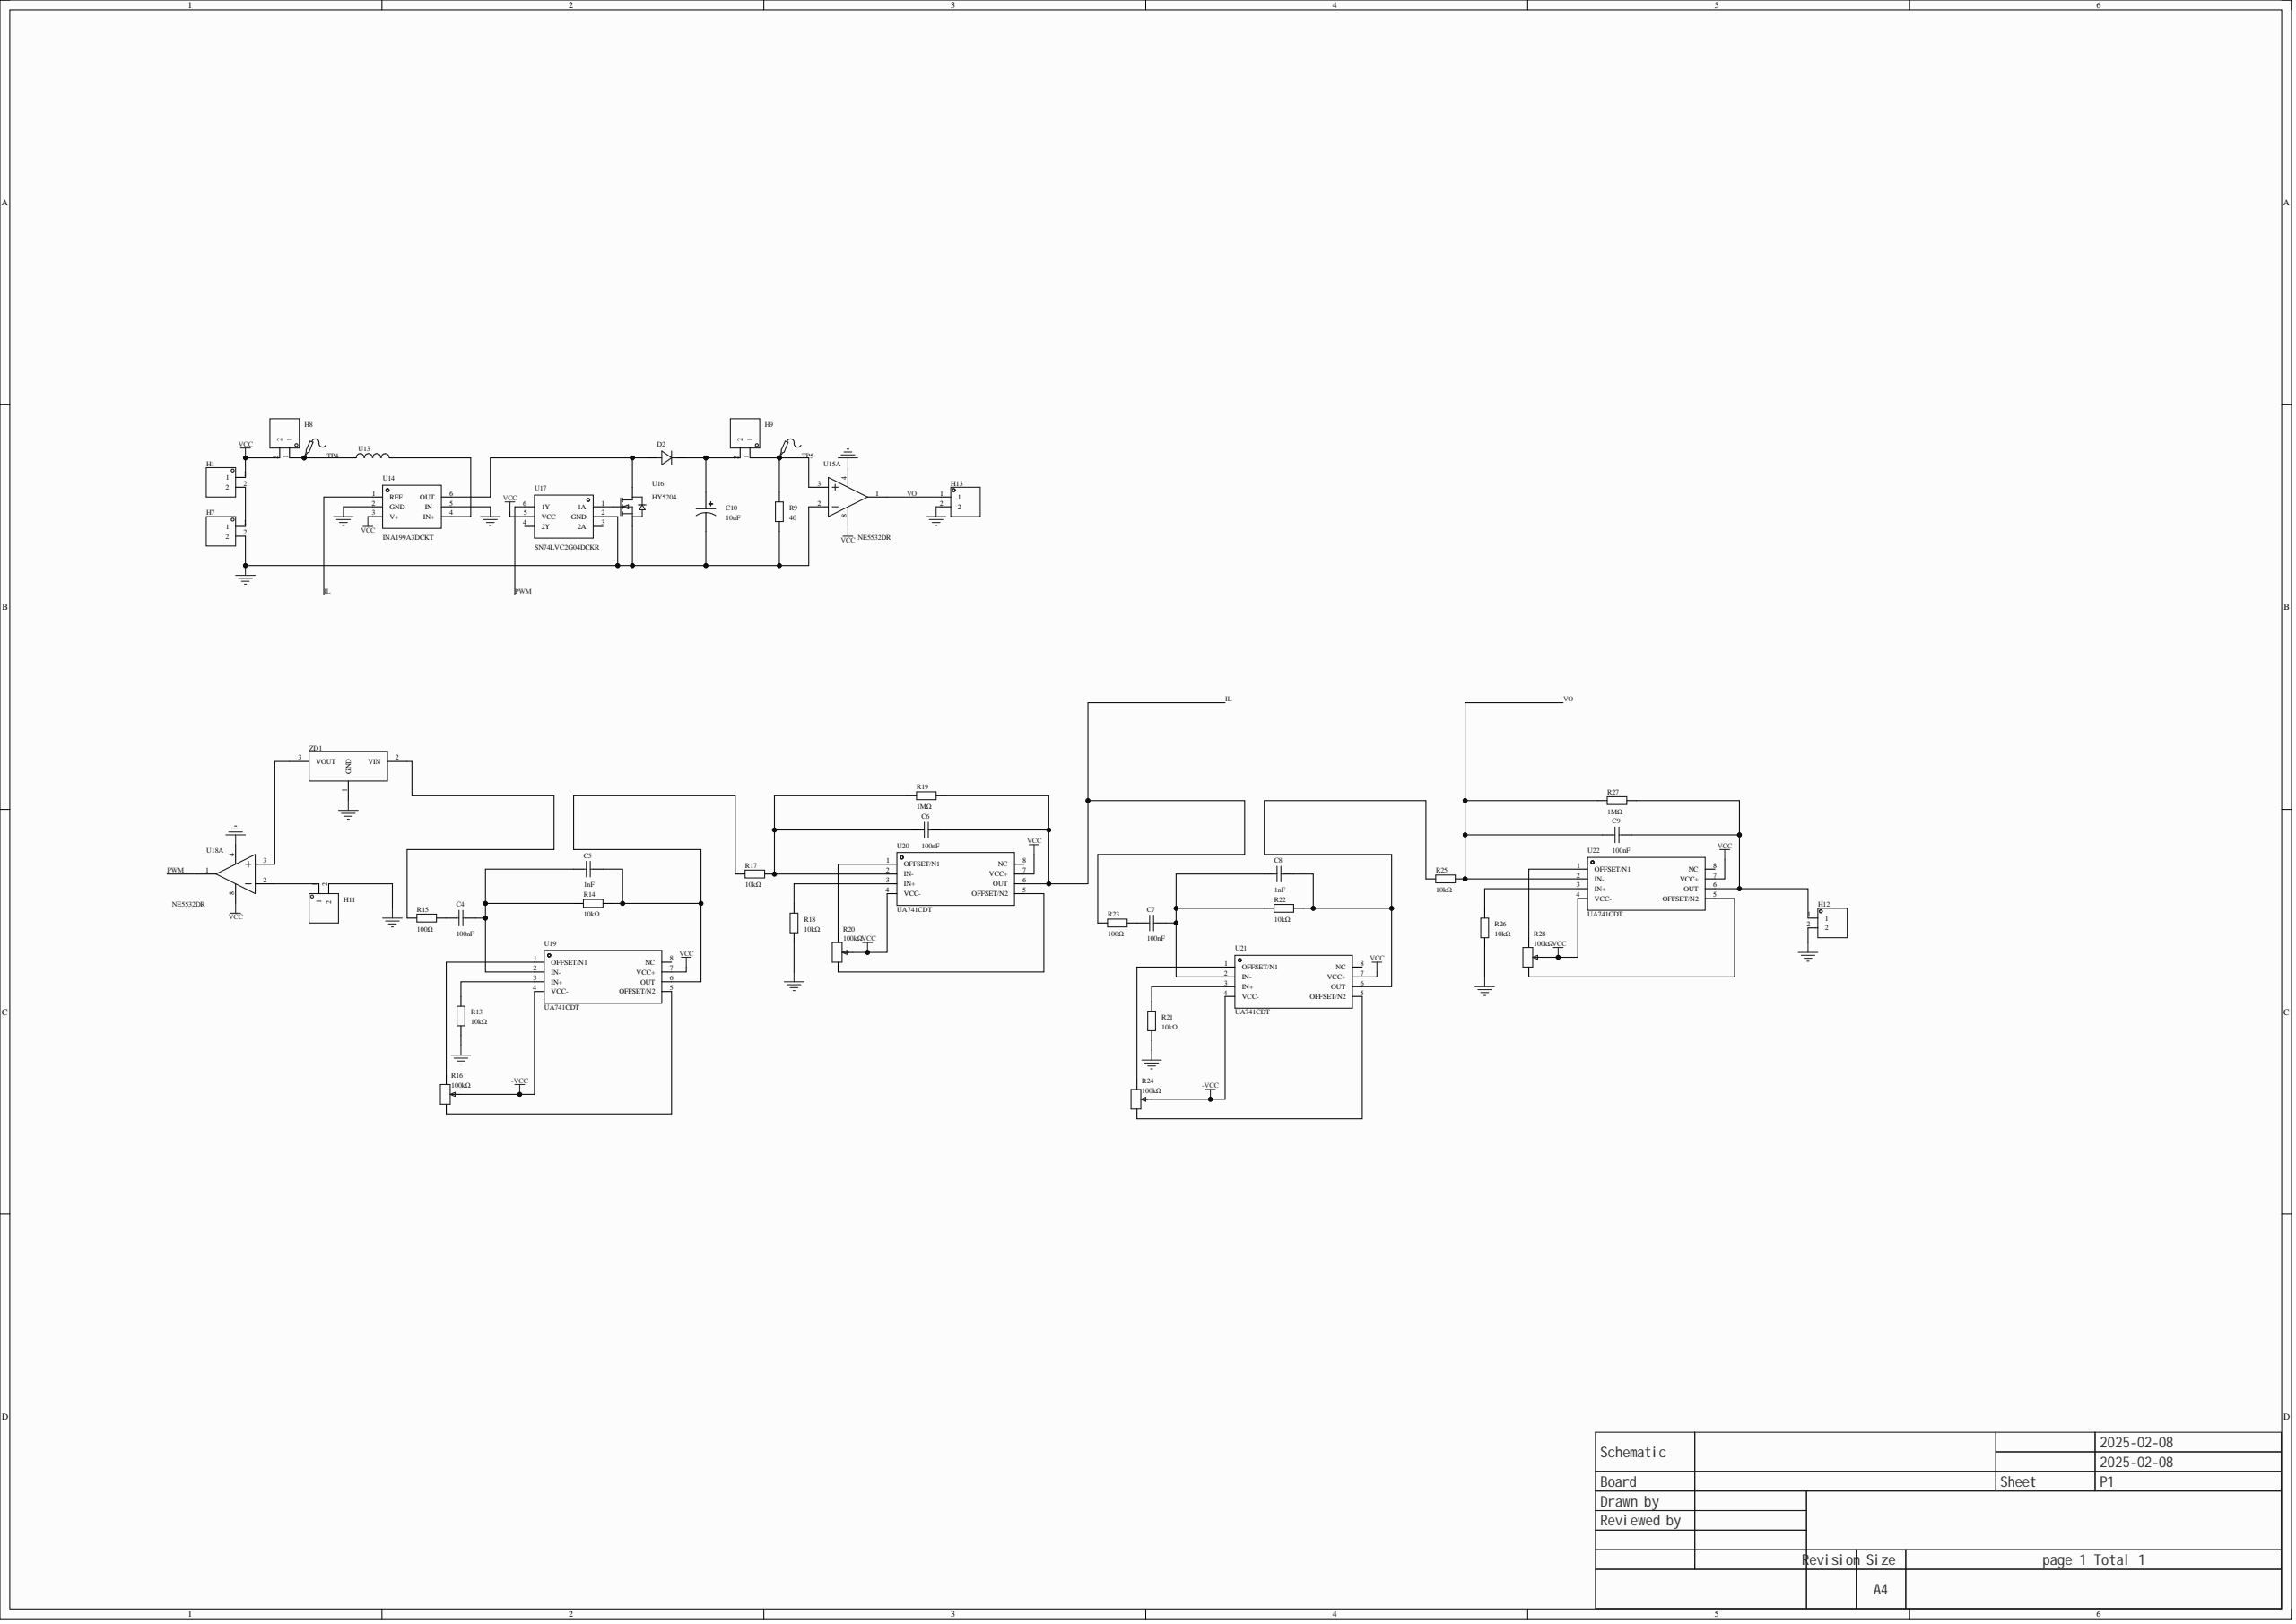Circuit board | Altium Designer | 45 parts | 36 nets
Bill of materials:
Comment,Description,Designator,Footprint,LibRef,Quantity
"100nF","Capacitance: 100nF; Tolerance: ±10%; Rated voltage: 50V; Dielectric (temperature coefficient): X7R;","C4, C6, C7, C9","C0805","CC0805KRX7R9BB104","4"
"1nF","Capacitance: 100nF; Tolerance: ±10%; Rated voltage: 50V; Dielectric (temperature coefficient): X7R;","C5, C8","C0805","CC0805KRX7R9BB104","2"
"10uF","Capacitance: 10uF; Tolerance: ±20%; Rated voltage: 10V; Ripple current: 16mA@120Hz;","C10","CAP-TH_BD4.0-P1.50-D0.8-FD","10MS510MEFC4X5","1"
"","","D2","DO_1N4007","D_1N4007A","1"
"","","H1, H7, H8, H9, H11, H12, H13","HDR-TH_2P-P2.54-V-M-1","HDR-M_2.54_1x2P","7"
"40","","R9","Res_1/4W","Res_AXIAL-1/4W","1"
"10kΩ","Resistor type: thick film resistor; Resistance: 10kΩ; Tolerance: ±1%; Power: 125mW; Max working voltage: 150V; Temperature coefficient: ±100ppm/?;","R13, R14, R17, R18, R21, R22, R25, R26","R0805","0805W8F1002T5E_C17414","8"
"100Ω","Resistor type: thick film resistor; Resistance: 10kΩ; Tolerance: ±1%; Power: 125mW; Max working voltage: 150V; Temperature coefficient: ±100ppm/?;","R15, R23","R0805","0805W8F1002T5E_C17414","2"
"100kΩ","Resistance: 200Ω; Tolerance: ±25%;","R16, R20, R24, R28","RES-ADJ-SMD_VG039NCH","VG039NCHXTB201","4"
"1MΩ","Resistor type: thick film resistor; Resistance: 10kΩ; Tolerance: ±1%; Power: 125mW; Max working voltage: 150V; Temperature coefficient: ±100ppm/?;","R19, R27","R0805","0805W8F1002T5E_C17414","2"
"","Test Point","TP4, TP5","Test-Point-0.5mm","Test-Point","2"
"Power inductor (SMD), CKST0502-10uH/M, 10uH, ±20%, 3A, package 5.7mm*5.1mm*2.0mm, Cenke, RoHS","","U13","IND-SMD_L5.7-W5.1","功率电感(贴片),CKST0502-10uH/M,10uH,±20%,3A,封装5.7mm*5.1mm*2.0mm,岑科,RoHS","1"
"INA199A3DCKT","26V bidirectional current sense amplifier 6-SC70 -40 to 125","U14","SC-70-6_L2.1-W1.3-P0.65-LS2.1-BR","INA199A3DCKT","1"
"NE5532DR","","U15, U18","SOIC-8_L4.9-W3.9-P1.27-LS6.0-BL","NE5532DR","2"
"HY5204","","U16","TO-247-3_L15.8-W5.0-P5.44-L-1","HY5204","1"
"SN74LVC2G04DCKR","Input type: -; Supply voltage: 1.65V~5.5V; Supply current (max): 10uA; Circuits: 2; Max propagation delay (tpd): 3.2ns@5V,50pF;","U17","SOT-363_L2.0-W1.3-P0.65-LS2.1-BR","SN74LVC2G04DCKR","1"
"UA741CDT","","U19, U20, U21, U22","SOIC-8_L4.9-W3.9-P1.27-LS6.0-BL","UA741CDT","4"
"","","ZD1","SOT-89-3_L4.5-W2.5-P1.50-LS4.2-BR","HT7233SOT89三端稳压300MA3.3VLDO稳压器","1"
Netlist (Protel format):
[
C4
C0805
100nF



]
[
C5
C0805
1nF



]
[
C6
C0805
100nF



]
[
C7
C0805
100nF



]
[
C8
C0805
1nF



]
[
C9
C0805
100nF



]
[
C10
CAP-TH_BD4.0-P1.50-D0.8-FD
10uF



]
[
D2
DO_1N4007




]
[
H1
HDR-TH_2P-P2.54-V-M-1




]
[
H7
HDR-TH_2P-P2.54-V-M-1




]
[
H8
HDR-TH_2P-P2.54-V-M-1




]
[
H9
HDR-TH_2P-P2.54-V-M-1




]
[
H11
HDR-TH_2P-P2.54-V-M-1




]
[
H12
HDR-TH_2P-P2.54-V-M-1




]
[
H13
HDR-TH_2P-P2.54-V-M-1




]
[
R9
Res_1/4W
40



]
[
R13
R0805
10kΩ



]
[
R14
R0805
10kΩ



]
[
R15
R0805
100Ω



]
[
R16
RES-ADJ-SMD_VG039NCH
100kΩ



]
[
R17
R0805
10kΩ



]
[
R18
R0805
10kΩ



]
[
R19
R0805
1MΩ



]
[
R20
RES-ADJ-SMD_VG039NCH
100kΩ



]
[
R21
R0805
10kΩ



]
[
R22
R0805
10kΩ



]
[
R23
R0805
100Ω



]
[
R24
RES-ADJ-SMD_VG039NCH
100kΩ



]
[
R25
R0805
10kΩ



]
[
R26
R0805
10kΩ



]
[
R27
R0805
1MΩ



]
[
R28
RES-ADJ-SMD_VG039NCH
100kΩ



]
[
TP4
Test-Point-0.5mm




]
[
TP5
Test-Point-0.5mm




]
[
U13
IND-SMD_L5.7-W5.1
Power inductor (SMD), CKST0502-10uH/M, 10uH, ±20%, 3A, package 5.7mm*5.1mm*2.0mm, Cenke, RoHS



]
[
U14
SC-70-6_L2.1-W1.3-P0.65-LS2.1-BR
INA199A3DCKT



]
[
U15
SOIC-8_L4.9-W3.9-P1.27-LS6.0-BL
NE5532DR



]
[
U16
TO-247-3_L15.8-W5.0-P5.44-L-1
HY5204



]
[
U17
SOT-363_L2.0-W1.3-P0.65-LS2.1-BR
SN74LVC2G04DCKR



]
[
U18
SOIC-8_L4.9-W3.9-P1.27-LS6.0-BL
NE5532DR



]
[
U19
SOIC-8_L4.9-W3.9-P1.27-LS6.0-BL
UA741CDT



]
[
U20
SOIC-8_L4.9-W3.9-P1.27-LS6.0-BL
UA741CDT



]
[
U21
SOIC-8_L4.9-W3.9-P1.27-LS6.0-BL
UA741CDT



]
[
U22
SOIC-8_L4.9-W3.9-P1.27-LS6.0-BL
UA741CDT



]
[
ZD1
SOT-89-3_L4.5-W2.5-P1.50-LS4.2-BR




]
(
VO
C9-1
H13-1
R25-2
R27-1
U15-1
U22-2
)
(
VCC
H1-1
H8-2
U14-3
U15-8
U17-5
U18-8
U19-7
U20-7
U21-7
U22-7
)
(
PWM
U17-6
U18-1
)
(
NetU18_3
U18-3
ZD1-3
)
(
NetU16_1
U16-1
U17-1
)
(
NetU13_2
U13-2
U14-4
)
(
NetR28_3
R28-3
U22-1
)
(
NetR28_1
R28-1
U22-5
)
(
NetR26_2
R26-2
U22-3
)
(
NetR24_3
R24-3
U21-5
)
(
NetR24_1
R24-1
U21-1
)
(
NetR21_2
R21-2
U21-3
)
(
NetR20_3
R20-3
U20-1
)
(
NetR20_1
R20-1
U20-5
)
(
NetR18_2
R18-2
U20-3
)
(
NetR16_3
R16-3
U19-5
)
(
NetR16_1
R16-1
U19-1
)
(
NetR15_1
R15-1
ZD1-2
)
(
NetR13_2
R13-2
U19-3
)
(
NetH11_1
H11-1
U18-2
)
(
NetH9_1
H9-1
R9-2
TP5-1
U15-3
)
(
NetH8_1
H8-1
TP4-1
U13-1
)
(
NetH1_2
H1-2
H7-1
)
(
NetD2_2
D2-2
U14-6
U16-2
)
(
NetC10_1
C10-1
D2-1
H9-2
)
(
NetC9_2
C9-2
H12-1
R27-2
U22-6
)
(
NetC8_2
C8-2
R22-2
R25-1
U21-6
)
(
NetC7_2
C7-2
C8-1
R22-1
U21-2
)
(
NetC7_1
C7-1
R23-2
)
(
NetC6_1
C6-1
R17-2
R19-1
U20-2
)
(
NetC5_2
C5-2
R14-2
R17-1
U19-6
)
(
NetC4_2
C4-2
C5-1
R14-1
U19-2
)
(
NetC4_1
C4-1
R15-2
)
(
IL
C6-2
R19-2
R23-1
U14-1
U20-6
)
(
GND
C10-2
H7-2
H11-2
H12-2
H13-2
R9-1
R13-1
R18-1
R21-1
R26-1
U14-2
U14-5
U15-2
U15-4
U16-3
U17-2
U18-4
ZD1-1
)
(
-VCC
R16-2
R20-2
R24-2
R28-2
U19-4
U20-4
U21-4
U22-4
)